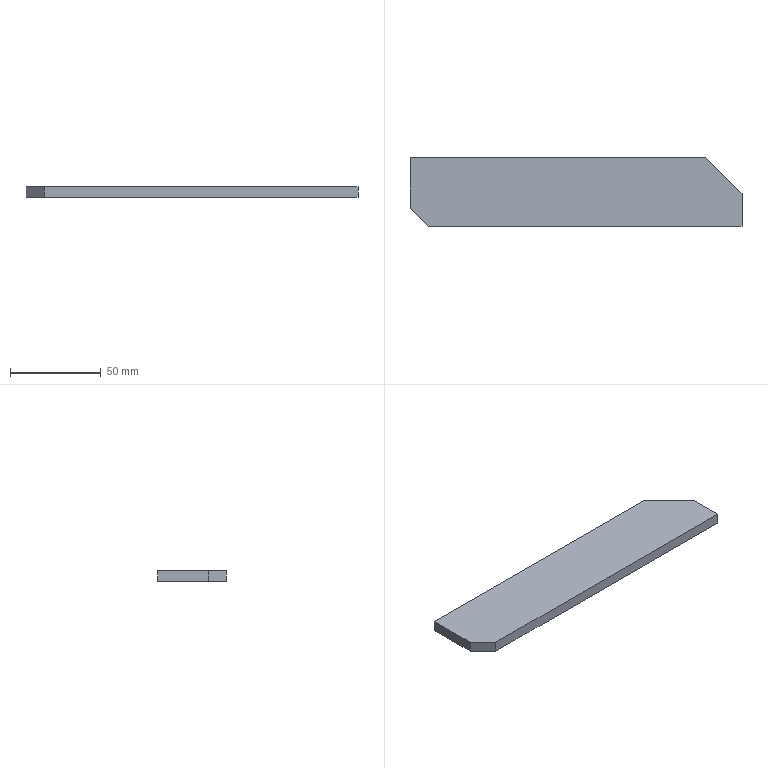Part | STEP file | [03]-10 | 1 solid | 8 faces | box 183 x 38 x 6 mm | volume 40224 mm3 | plane 8
STEP:
#1=CARTESIAN_POINT('',(0.,0.,0.));
#2=DIRECTION('',(0.,0.,1.));
#3=DIRECTION('',(1.,0.,0.));
#4=AXIS2_PLACEMENT_3D('',#1,#2,#3);
#5=CARTESIAN_POINT('',(0.,10.,6.));
#6=VERTEX_POINT('',#5);
#7=CARTESIAN_POINT('',(0.,38.,6.));
#8=VERTEX_POINT('',#7);
#9=CARTESIAN_POINT('',(0.,19.,6.));
#10=DIRECTION('',(0.,1.,0.));
#11=VECTOR('',#10,1.);
#12=LINE('',#9,#11);
#13=CARTESIAN_POINT('',(91.5,19.,6.));
#14=DIRECTION('',(0.,0.,1.));
#15=DIRECTION('',(-1.,0.,0.));
#16=AXIS2_PLACEMENT_3D('',#13,#14,#15);
#17=PLANE('',#16);
#18=CARTESIAN_POINT('',(91.5,0.));
#19=DIRECTION('',(0.,-1.));
#20=VECTOR('',#19,1.);
#21=LINE('',#18,#20);
#22=(GEOMETRIC_REPRESENTATION_CONTEXT(2)PARAMETRIC_REPRESENTATION_CONTEXT()REPRESENTATION_CONTEXT('',''));
#23=DEFINITIONAL_REPRESENTATION('',(#21),#22);
#24=PCURVE('',#17,#23);
#25=CARTESIAN_POINT('',(0.,19.,0.));
#26=DIRECTION('',(-1.,0.,0.));
#27=DIRECTION('',(0.,0.,-1.));
#28=AXIS2_PLACEMENT_3D('',#25,#26,#27);
#29=PLANE('',#28);
#30=CARTESIAN_POINT('',(-6.,0.));
#31=DIRECTION('',(0.,-1.));
#32=VECTOR('',#31,1.);
#33=LINE('',#30,#32);
#34=(GEOMETRIC_REPRESENTATION_CONTEXT(2)PARAMETRIC_REPRESENTATION_CONTEXT()REPRESENTATION_CONTEXT('',''));
#35=DEFINITIONAL_REPRESENTATION('',(#33),#34);
#36=PCURVE('',#29,#35);
#37=SURFACE_CURVE('',#12,(#24,#36),.PCURVE_S1.);
#38=EDGE_CURVE('',#6,#8,#37,.T.);
#39=ORIENTED_EDGE('',*,*,#38,.F.);
#40=CARTESIAN_POINT('',(10.,0.,6.));
#41=VERTEX_POINT('',#40);
#42=CARTESIAN_POINT('',(41.25,-31.25,6.));
#43=DIRECTION('',(0.7071,-0.7071,0.));
#44=VECTOR('',#43,1.);
#45=LINE('',#42,#44);
#46=CARTESIAN_POINT('',(50.25,50.25));
#47=DIRECTION('',(-0.7071,0.7071));
#48=VECTOR('',#47,1.);
#49=LINE('',#46,#48);
#50=(GEOMETRIC_REPRESENTATION_CONTEXT(2)PARAMETRIC_REPRESENTATION_CONTEXT()REPRESENTATION_CONTEXT('',''));
#51=DEFINITIONAL_REPRESENTATION('',(#49),#50);
#52=PCURVE('',#17,#51);
#53=CARTESIAN_POINT('',(0.,10.,0.));
#54=DIRECTION('',(0.7071,0.7071,0.));
#55=DIRECTION('',(0.,0.,1.));
#56=AXIS2_PLACEMENT_3D('',#53,#54,#55);
#57=PLANE('',#56);
#58=CARTESIAN_POINT('',(6.,58.336));
#59=DIRECTION('',(0.,1.));
#60=VECTOR('',#59,1.);
#61=LINE('',#58,#60);
#62=(GEOMETRIC_REPRESENTATION_CONTEXT(2)PARAMETRIC_REPRESENTATION_CONTEXT()REPRESENTATION_CONTEXT('',''));
#63=DEFINITIONAL_REPRESENTATION('',(#61),#62);
#64=PCURVE('',#57,#63);
#65=SURFACE_CURVE('',#45,(#52,#64),.PCURVE_S1.);
#66=EDGE_CURVE('',#6,#41,#65,.T.);
#67=ORIENTED_EDGE('',*,*,#66,.T.);
#68=CARTESIAN_POINT('',(183.,0.,6.));
#69=VERTEX_POINT('',#68);
#70=CARTESIAN_POINT('',(91.5,0.,6.));
#71=DIRECTION('',(-1.,0.,0.));
#72=VECTOR('',#71,1.);
#73=LINE('',#70,#72);
#74=CARTESIAN_POINT('',(0.,19.));
#75=DIRECTION('',(1.,0.));
#76=VECTOR('',#75,1.);
#77=LINE('',#74,#76);
#78=(GEOMETRIC_REPRESENTATION_CONTEXT(2)PARAMETRIC_REPRESENTATION_CONTEXT()REPRESENTATION_CONTEXT('',''));
#79=DEFINITIONAL_REPRESENTATION('',(#77),#78);
#80=PCURVE('',#17,#79);
#81=CARTESIAN_POINT('',(91.5,0.,0.));
#82=DIRECTION('',(0.,-1.,0.));
#83=DIRECTION('',(0.,0.,1.));
#84=AXIS2_PLACEMENT_3D('',#81,#82,#83);
#85=PLANE('',#84);
#86=CARTESIAN_POINT('',(6.,0.));
#87=DIRECTION('',(0.,1.));
#88=VECTOR('',#87,1.);
#89=LINE('',#86,#88);
#90=(GEOMETRIC_REPRESENTATION_CONTEXT(2)PARAMETRIC_REPRESENTATION_CONTEXT()REPRESENTATION_CONTEXT('',''));
#91=DEFINITIONAL_REPRESENTATION('',(#89),#90);
#92=PCURVE('',#85,#91);
#93=SURFACE_CURVE('',#73,(#80,#92),.PCURVE_S1.);
#94=EDGE_CURVE('',#69,#41,#93,.T.);
#95=ORIENTED_EDGE('',*,*,#94,.F.);
#96=CARTESIAN_POINT('',(183.,18.,6.));
#97=VERTEX_POINT('',#96);
#98=CARTESIAN_POINT('',(183.,19.,6.));
#99=DIRECTION('',(0.,-1.,0.));
#100=VECTOR('',#99,1.);
#101=LINE('',#98,#100);
#102=CARTESIAN_POINT('',(-91.5,0.));
#103=DIRECTION('',(0.,1.));
#104=VECTOR('',#103,1.);
#105=LINE('',#102,#104);
#106=(GEOMETRIC_REPRESENTATION_CONTEXT(2)PARAMETRIC_REPRESENTATION_CONTEXT()REPRESENTATION_CONTEXT('',''));
#107=DEFINITIONAL_REPRESENTATION('',(#105),#106);
#108=PCURVE('',#17,#107);
#109=CARTESIAN_POINT('',(183.,19.,0.));
#110=DIRECTION('',(1.,0.,0.));
#111=DIRECTION('',(0.,0.,1.));
#112=AXIS2_PLACEMENT_3D('',#109,#110,#111);
#113=PLANE('',#112);
#114=CARTESIAN_POINT('',(6.,0.));
#115=DIRECTION('',(0.,1.));
#116=VECTOR('',#115,1.);
#117=LINE('',#114,#116);
#118=(GEOMETRIC_REPRESENTATION_CONTEXT(2)PARAMETRIC_REPRESENTATION_CONTEXT()REPRESENTATION_CONTEXT('',''));
#119=DEFINITIONAL_REPRESENTATION('',(#117),#118);
#120=PCURVE('',#113,#119);
#121=SURFACE_CURVE('',#101,(#108,#120),.PCURVE_S1.);
#122=EDGE_CURVE('',#97,#69,#121,.T.);
#123=ORIENTED_EDGE('',*,*,#122,.F.);
#124=CARTESIAN_POINT('',(163.,38.,6.));
#125=VERTEX_POINT('',#124);
#126=CARTESIAN_POINT('',(136.75,64.25,6.));
#127=DIRECTION('',(-0.7071,0.7071,0.));
#128=VECTOR('',#127,1.);
#129=LINE('',#126,#128);
#130=CARTESIAN_POINT('',(-45.25,-45.25));
#131=DIRECTION('',(0.7071,-0.7071));
#132=VECTOR('',#131,1.);
#133=LINE('',#130,#132);
#134=(GEOMETRIC_REPRESENTATION_CONTEXT(2)PARAMETRIC_REPRESENTATION_CONTEXT()REPRESENTATION_CONTEXT('',''));
#135=DEFINITIONAL_REPRESENTATION('',(#133),#134);
#136=PCURVE('',#17,#135);
#137=CARTESIAN_POINT('',(183.,18.,0.));
#138=DIRECTION('',(-0.7071,-0.7071,0.));
#139=DIRECTION('',(0.,0.,1.));
#140=AXIS2_PLACEMENT_3D('',#137,#138,#139);
#141=PLANE('',#140);
#142=CARTESIAN_POINT('',(6.,65.407));
#143=DIRECTION('',(0.,1.));
#144=VECTOR('',#143,1.);
#145=LINE('',#142,#144);
#146=(GEOMETRIC_REPRESENTATION_CONTEXT(2)PARAMETRIC_REPRESENTATION_CONTEXT()REPRESENTATION_CONTEXT('',''));
#147=DEFINITIONAL_REPRESENTATION('',(#145),#146);
#148=PCURVE('',#141,#147);
#149=SURFACE_CURVE('',#129,(#136,#148),.PCURVE_S1.);
#150=EDGE_CURVE('',#97,#125,#149,.T.);
#151=ORIENTED_EDGE('',*,*,#150,.T.);
#152=CARTESIAN_POINT('',(91.5,38.,6.));
#153=DIRECTION('',(1.,0.,0.));
#154=VECTOR('',#153,1.);
#155=LINE('',#152,#154);
#156=CARTESIAN_POINT('',(0.,-19.));
#157=DIRECTION('',(-1.,0.));
#158=VECTOR('',#157,1.);
#159=LINE('',#156,#158);
#160=(GEOMETRIC_REPRESENTATION_CONTEXT(2)PARAMETRIC_REPRESENTATION_CONTEXT()REPRESENTATION_CONTEXT('',''));
#161=DEFINITIONAL_REPRESENTATION('',(#159),#160);
#162=PCURVE('',#17,#161);
#163=CARTESIAN_POINT('',(91.5,38.,0.));
#164=DIRECTION('',(0.,1.,0.));
#165=DIRECTION('',(0.,0.,-1.));
#166=AXIS2_PLACEMENT_3D('',#163,#164,#165);
#167=PLANE('',#166);
#168=CARTESIAN_POINT('',(-6.,0.));
#169=DIRECTION('',(0.,-1.));
#170=VECTOR('',#169,1.);
#171=LINE('',#168,#170);
#172=(GEOMETRIC_REPRESENTATION_CONTEXT(2)PARAMETRIC_REPRESENTATION_CONTEXT()REPRESENTATION_CONTEXT('',''));
#173=DEFINITIONAL_REPRESENTATION('',(#171),#172);
#174=PCURVE('',#167,#173);
#175=SURFACE_CURVE('',#155,(#162,#174),.PCURVE_S1.);
#176=EDGE_CURVE('',#8,#125,#175,.T.);
#177=ORIENTED_EDGE('',*,*,#176,.F.);
#178=EDGE_LOOP('',(#39,#67,#95,#123,#151,#177));
#179=FACE_BOUND('',#178,.T.);
#180=ADVANCED_FACE('',(#179),#17,.T.);
#181=ORIENTED_EDGE('',*,*,#176,.T.);
#182=CARTESIAN_POINT('',(163.,38.,0.));
#183=VERTEX_POINT('',#182);
#184=CARTESIAN_POINT('',(163.,38.,0.));
#185=DIRECTION('',(0.,0.,-1.));
#186=VECTOR('',#185,1.);
#187=LINE('',#184,#186);
#188=CARTESIAN_POINT('',(0.,-71.5));
#189=DIRECTION('',(1.,0.));
#190=VECTOR('',#189,1.);
#191=LINE('',#188,#190);
#192=(GEOMETRIC_REPRESENTATION_CONTEXT(2)PARAMETRIC_REPRESENTATION_CONTEXT()REPRESENTATION_CONTEXT('',''));
#193=DEFINITIONAL_REPRESENTATION('',(#191),#192);
#194=PCURVE('',#167,#193);
#195=CARTESIAN_POINT('',(0.,28.284));
#196=DIRECTION('',(-1.,0.));
#197=VECTOR('',#196,1.);
#198=LINE('',#195,#197);
#199=(GEOMETRIC_REPRESENTATION_CONTEXT(2)PARAMETRIC_REPRESENTATION_CONTEXT()REPRESENTATION_CONTEXT('',''));
#200=DEFINITIONAL_REPRESENTATION('',(#198),#199);
#201=PCURVE('',#141,#200);
#202=SURFACE_CURVE('',#187,(#194,#201),.PCURVE_S1.);
#203=EDGE_CURVE('',#125,#183,#202,.T.);
#204=ORIENTED_EDGE('',*,*,#203,.T.);
#205=CARTESIAN_POINT('',(0.,38.,0.));
#206=VERTEX_POINT('',#205);
#207=CARTESIAN_POINT('',(91.5,38.,0.));
#208=DIRECTION('',(-1.,0.,0.));
#209=VECTOR('',#208,1.);
#210=LINE('',#207,#209);
#211=CARTESIAN_POINT('',(0.,0.));
#212=DIRECTION('',(0.,1.));
#213=VECTOR('',#212,1.);
#214=LINE('',#211,#213);
#215=(GEOMETRIC_REPRESENTATION_CONTEXT(2)PARAMETRIC_REPRESENTATION_CONTEXT()REPRESENTATION_CONTEXT('',''));
#216=DEFINITIONAL_REPRESENTATION('',(#214),#215);
#217=PCURVE('',#167,#216);
#218=CARTESIAN_POINT('',(91.5,19.,0.));
#219=DIRECTION('',(0.,0.,-1.));
#220=DIRECTION('',(1.,0.,0.));
#221=AXIS2_PLACEMENT_3D('',#218,#219,#220);
#222=PLANE('',#221);
#223=CARTESIAN_POINT('',(0.,-19.));
#224=DIRECTION('',(-1.,0.));
#225=VECTOR('',#224,1.);
#226=LINE('',#223,#225);
#227=(GEOMETRIC_REPRESENTATION_CONTEXT(2)PARAMETRIC_REPRESENTATION_CONTEXT()REPRESENTATION_CONTEXT('',''));
#228=DEFINITIONAL_REPRESENTATION('',(#226),#227);
#229=PCURVE('',#222,#228);
#230=SURFACE_CURVE('',#210,(#217,#229),.PCURVE_S1.);
#231=EDGE_CURVE('',#183,#206,#230,.T.);
#232=ORIENTED_EDGE('',*,*,#231,.T.);
#233=CARTESIAN_POINT('',(0.,38.,0.));
#234=DIRECTION('',(0.,0.,1.));
#235=VECTOR('',#234,1.);
#236=LINE('',#233,#235);
#237=CARTESIAN_POINT('',(0.,91.5));
#238=DIRECTION('',(-1.,0.));
#239=VECTOR('',#238,1.);
#240=LINE('',#237,#239);
#241=(GEOMETRIC_REPRESENTATION_CONTEXT(2)PARAMETRIC_REPRESENTATION_CONTEXT()REPRESENTATION_CONTEXT('',''));
#242=DEFINITIONAL_REPRESENTATION('',(#240),#241);
#243=PCURVE('',#167,#242);
#244=CARTESIAN_POINT('',(0.,-19.));
#245=DIRECTION('',(-1.,0.));
#246=VECTOR('',#245,1.);
#247=LINE('',#244,#246);
#248=(GEOMETRIC_REPRESENTATION_CONTEXT(2)PARAMETRIC_REPRESENTATION_CONTEXT()REPRESENTATION_CONTEXT('',''));
#249=DEFINITIONAL_REPRESENTATION('',(#247),#248);
#250=PCURVE('',#29,#249);
#251=SURFACE_CURVE('',#236,(#243,#250),.PCURVE_S1.);
#252=EDGE_CURVE('',#206,#8,#251,.T.);
#253=ORIENTED_EDGE('',*,*,#252,.T.);
#254=EDGE_LOOP('',(#181,#204,#232,#253));
#255=FACE_BOUND('',#254,.T.);
#256=ADVANCED_FACE('',(#255),#167,.T.);
#257=CARTESIAN_POINT('',(183.,0.,0.));
#258=VERTEX_POINT('',#257);
#259=CARTESIAN_POINT('',(183.,18.,0.));
#260=VERTEX_POINT('',#259);
#261=CARTESIAN_POINT('',(183.,19.,0.));
#262=DIRECTION('',(0.,1.,0.));
#263=VECTOR('',#262,1.);
#264=LINE('',#261,#263);
#265=CARTESIAN_POINT('',(0.,0.));
#266=DIRECTION('',(0.,-1.));
#267=VECTOR('',#266,1.);
#268=LINE('',#265,#267);
#269=(GEOMETRIC_REPRESENTATION_CONTEXT(2)PARAMETRIC_REPRESENTATION_CONTEXT()REPRESENTATION_CONTEXT('',''));
#270=DEFINITIONAL_REPRESENTATION('',(#268),#269);
#271=PCURVE('',#113,#270);
#272=CARTESIAN_POINT('',(91.5,0.));
#273=DIRECTION('',(0.,-1.));
#274=VECTOR('',#273,1.);
#275=LINE('',#272,#274);
#276=(GEOMETRIC_REPRESENTATION_CONTEXT(2)PARAMETRIC_REPRESENTATION_CONTEXT()REPRESENTATION_CONTEXT('',''));
#277=DEFINITIONAL_REPRESENTATION('',(#275),#276);
#278=PCURVE('',#222,#277);
#279=SURFACE_CURVE('',#264,(#271,#278),.PCURVE_S1.);
#280=EDGE_CURVE('',#258,#260,#279,.T.);
#281=ORIENTED_EDGE('',*,*,#280,.T.);
#282=CARTESIAN_POINT('',(183.,18.,0.));
#283=DIRECTION('',(0.,0.,1.));
#284=VECTOR('',#283,1.);
#285=LINE('',#282,#284);
#286=CARTESIAN_POINT('',(0.,1.));
#287=DIRECTION('',(1.,0.));
#288=VECTOR('',#287,1.);
#289=LINE('',#286,#288);
#290=(GEOMETRIC_REPRESENTATION_CONTEXT(2)PARAMETRIC_REPRESENTATION_CONTEXT()REPRESENTATION_CONTEXT('',''));
#291=DEFINITIONAL_REPRESENTATION('',(#289),#290);
#292=PCURVE('',#113,#291);
#293=CARTESIAN_POINT('',(0.,0.));
#294=DIRECTION('',(1.,0.));
#295=VECTOR('',#294,1.);
#296=LINE('',#293,#295);
#297=(GEOMETRIC_REPRESENTATION_CONTEXT(2)PARAMETRIC_REPRESENTATION_CONTEXT()REPRESENTATION_CONTEXT('',''));
#298=DEFINITIONAL_REPRESENTATION('',(#296),#297);
#299=PCURVE('',#141,#298);
#300=SURFACE_CURVE('',#285,(#292,#299),.PCURVE_S1.);
#301=EDGE_CURVE('',#260,#97,#300,.T.);
#302=ORIENTED_EDGE('',*,*,#301,.T.);
#303=ORIENTED_EDGE('',*,*,#122,.T.);
#304=CARTESIAN_POINT('',(183.,0.,0.));
#305=DIRECTION('',(0.,0.,1.));
#306=VECTOR('',#305,1.);
#307=LINE('',#304,#306);
#308=CARTESIAN_POINT('',(0.,19.));
#309=DIRECTION('',(1.,0.));
#310=VECTOR('',#309,1.);
#311=LINE('',#308,#310);
#312=(GEOMETRIC_REPRESENTATION_CONTEXT(2)PARAMETRIC_REPRESENTATION_CONTEXT()REPRESENTATION_CONTEXT('',''));
#313=DEFINITIONAL_REPRESENTATION('',(#311),#312);
#314=PCURVE('',#113,#313);
#315=CARTESIAN_POINT('',(0.,-91.5));
#316=DIRECTION('',(1.,0.));
#317=VECTOR('',#316,1.);
#318=LINE('',#315,#317);
#319=(GEOMETRIC_REPRESENTATION_CONTEXT(2)PARAMETRIC_REPRESENTATION_CONTEXT()REPRESENTATION_CONTEXT('',''));
#320=DEFINITIONAL_REPRESENTATION('',(#318),#319);
#321=PCURVE('',#85,#320);
#322=SURFACE_CURVE('',#307,(#314,#321),.PCURVE_S1.);
#323=EDGE_CURVE('',#258,#69,#322,.T.);
#324=ORIENTED_EDGE('',*,*,#323,.F.);
#325=EDGE_LOOP('',(#281,#302,#303,#324));
#326=FACE_BOUND('',#325,.T.);
#327=ADVANCED_FACE('',(#326),#113,.T.);
#328=ORIENTED_EDGE('',*,*,#94,.T.);
#329=CARTESIAN_POINT('',(10.,0.,0.));
#330=VERTEX_POINT('',#329);
#331=CARTESIAN_POINT('',(10.,0.,0.));
#332=DIRECTION('',(0.,0.,-1.));
#333=VECTOR('',#332,1.);
#334=LINE('',#331,#333);
#335=CARTESIAN_POINT('',(0.,81.5));
#336=DIRECTION('',(-1.,0.));
#337=VECTOR('',#336,1.);
#338=LINE('',#335,#337);
#339=(GEOMETRIC_REPRESENTATION_CONTEXT(2)PARAMETRIC_REPRESENTATION_CONTEXT()REPRESENTATION_CONTEXT('',''));
#340=DEFINITIONAL_REPRESENTATION('',(#338),#339);
#341=PCURVE('',#85,#340);
#342=CARTESIAN_POINT('',(0.,14.142));
#343=DIRECTION('',(-1.,0.));
#344=VECTOR('',#343,1.);
#345=LINE('',#342,#344);
#346=(GEOMETRIC_REPRESENTATION_CONTEXT(2)PARAMETRIC_REPRESENTATION_CONTEXT()REPRESENTATION_CONTEXT('',''));
#347=DEFINITIONAL_REPRESENTATION('',(#345),#346);
#348=PCURVE('',#57,#347);
#349=SURFACE_CURVE('',#334,(#341,#348),.PCURVE_S1.);
#350=EDGE_CURVE('',#41,#330,#349,.T.);
#351=ORIENTED_EDGE('',*,*,#350,.T.);
#352=CARTESIAN_POINT('',(91.5,0.,0.));
#353=DIRECTION('',(1.,0.,0.));
#354=VECTOR('',#353,1.);
#355=LINE('',#352,#354);
#356=CARTESIAN_POINT('',(0.,0.));
#357=DIRECTION('',(0.,-1.));
#358=VECTOR('',#357,1.);
#359=LINE('',#356,#358);
#360=(GEOMETRIC_REPRESENTATION_CONTEXT(2)PARAMETRIC_REPRESENTATION_CONTEXT()REPRESENTATION_CONTEXT('',''));
#361=DEFINITIONAL_REPRESENTATION('',(#359),#360);
#362=PCURVE('',#85,#361);
#363=CARTESIAN_POINT('',(0.,19.));
#364=DIRECTION('',(1.,0.));
#365=VECTOR('',#364,1.);
#366=LINE('',#363,#365);
#367=(GEOMETRIC_REPRESENTATION_CONTEXT(2)PARAMETRIC_REPRESENTATION_CONTEXT()REPRESENTATION_CONTEXT('',''));
#368=DEFINITIONAL_REPRESENTATION('',(#366),#367);
#369=PCURVE('',#222,#368);
#370=SURFACE_CURVE('',#355,(#362,#369),.PCURVE_S1.);
#371=EDGE_CURVE('',#330,#258,#370,.T.);
#372=ORIENTED_EDGE('',*,*,#371,.T.);
#373=ORIENTED_EDGE('',*,*,#323,.T.);
#374=EDGE_LOOP('',(#328,#351,#372,#373));
#375=FACE_BOUND('',#374,.T.);
#376=ADVANCED_FACE('',(#375),#85,.T.);
#377=ORIENTED_EDGE('',*,*,#371,.F.);
#378=CARTESIAN_POINT('',(0.,10.,0.));
#379=VERTEX_POINT('',#378);
#380=CARTESIAN_POINT('',(41.25,-31.25,0.));
#381=DIRECTION('',(-0.7071,0.7071,0.));
#382=VECTOR('',#381,1.);
#383=LINE('',#380,#382);
#384=CARTESIAN_POINT('',(-50.25,50.25));
#385=DIRECTION('',(-0.7071,-0.7071));
#386=VECTOR('',#385,1.);
#387=LINE('',#384,#386);
#388=(GEOMETRIC_REPRESENTATION_CONTEXT(2)PARAMETRIC_REPRESENTATION_CONTEXT()REPRESENTATION_CONTEXT('',''));
#389=DEFINITIONAL_REPRESENTATION('',(#387),#388);
#390=PCURVE('',#222,#389);
#391=CARTESIAN_POINT('',(0.,58.336));
#392=DIRECTION('',(0.,-1.));
#393=VECTOR('',#392,1.);
#394=LINE('',#391,#393);
#395=(GEOMETRIC_REPRESENTATION_CONTEXT(2)PARAMETRIC_REPRESENTATION_CONTEXT()REPRESENTATION_CONTEXT('',''));
#396=DEFINITIONAL_REPRESENTATION('',(#394),#395);
#397=PCURVE('',#57,#396);
#398=SURFACE_CURVE('',#383,(#390,#397),.PCURVE_S1.);
#399=EDGE_CURVE('',#330,#379,#398,.T.);
#400=ORIENTED_EDGE('',*,*,#399,.T.);
#401=CARTESIAN_POINT('',(0.,19.,0.));
#402=DIRECTION('',(0.,-1.,0.));
#403=VECTOR('',#402,1.);
#404=LINE('',#401,#403);
#405=CARTESIAN_POINT('',(-91.5,0.));
#406=DIRECTION('',(0.,1.));
#407=VECTOR('',#406,1.);
#408=LINE('',#405,#407);
#409=(GEOMETRIC_REPRESENTATION_CONTEXT(2)PARAMETRIC_REPRESENTATION_CONTEXT()REPRESENTATION_CONTEXT('',''));
#410=DEFINITIONAL_REPRESENTATION('',(#408),#409);
#411=PCURVE('',#222,#410);
#412=CARTESIAN_POINT('',(0.,0.));
#413=DIRECTION('',(0.,1.));
#414=VECTOR('',#413,1.);
#415=LINE('',#412,#414);
#416=(GEOMETRIC_REPRESENTATION_CONTEXT(2)PARAMETRIC_REPRESENTATION_CONTEXT()REPRESENTATION_CONTEXT('',''));
#417=DEFINITIONAL_REPRESENTATION('',(#415),#416);
#418=PCURVE('',#29,#417);
#419=SURFACE_CURVE('',#404,(#411,#418),.PCURVE_S1.);
#420=EDGE_CURVE('',#206,#379,#419,.T.);
#421=ORIENTED_EDGE('',*,*,#420,.F.);
#422=ORIENTED_EDGE('',*,*,#231,.F.);
#423=CARTESIAN_POINT('',(136.75,64.25,0.));
#424=DIRECTION('',(0.7071,-0.7071,0.));
#425=VECTOR('',#424,1.);
#426=LINE('',#423,#425);
#427=CARTESIAN_POINT('',(45.25,-45.25));
#428=DIRECTION('',(0.7071,0.7071));
#429=VECTOR('',#428,1.);
#430=LINE('',#427,#429);
#431=(GEOMETRIC_REPRESENTATION_CONTEXT(2)PARAMETRIC_REPRESENTATION_CONTEXT()REPRESENTATION_CONTEXT('',''));
#432=DEFINITIONAL_REPRESENTATION('',(#430),#431);
#433=PCURVE('',#222,#432);
#434=CARTESIAN_POINT('',(0.,65.407));
#435=DIRECTION('',(0.,-1.));
#436=VECTOR('',#435,1.);
#437=LINE('',#434,#436);
#438=(GEOMETRIC_REPRESENTATION_CONTEXT(2)PARAMETRIC_REPRESENTATION_CONTEXT()REPRESENTATION_CONTEXT('',''));
#439=DEFINITIONAL_REPRESENTATION('',(#437),#438);
#440=PCURVE('',#141,#439);
#441=SURFACE_CURVE('',#426,(#433,#440),.PCURVE_S1.);
#442=EDGE_CURVE('',#183,#260,#441,.T.);
#443=ORIENTED_EDGE('',*,*,#442,.T.);
#444=ORIENTED_EDGE('',*,*,#280,.F.);
#445=EDGE_LOOP('',(#377,#400,#421,#422,#443,#444));
#446=FACE_BOUND('',#445,.T.);
#447=ADVANCED_FACE('',(#446),#222,.T.);
#448=ORIENTED_EDGE('',*,*,#420,.T.);
#449=CARTESIAN_POINT('',(0.,10.,0.));
#450=DIRECTION('',(0.,0.,1.));
#451=VECTOR('',#450,1.);
#452=LINE('',#449,#451);
#453=CARTESIAN_POINT('',(0.,9.));
#454=DIRECTION('',(-1.,0.));
#455=VECTOR('',#454,1.);
#456=LINE('',#453,#455);
#457=(GEOMETRIC_REPRESENTATION_CONTEXT(2)PARAMETRIC_REPRESENTATION_CONTEXT()REPRESENTATION_CONTEXT('',''));
#458=DEFINITIONAL_REPRESENTATION('',(#456),#457);
#459=PCURVE('',#29,#458);
#460=CARTESIAN_POINT('',(0.,0.));
#461=DIRECTION('',(1.,0.));
#462=VECTOR('',#461,1.);
#463=LINE('',#460,#462);
#464=(GEOMETRIC_REPRESENTATION_CONTEXT(2)PARAMETRIC_REPRESENTATION_CONTEXT()REPRESENTATION_CONTEXT('',''));
#465=DEFINITIONAL_REPRESENTATION('',(#463),#464);
#466=PCURVE('',#57,#465);
#467=SURFACE_CURVE('',#452,(#459,#466),.PCURVE_S1.);
#468=EDGE_CURVE('',#379,#6,#467,.T.);
#469=ORIENTED_EDGE('',*,*,#468,.T.);
#470=ORIENTED_EDGE('',*,*,#38,.T.);
#471=ORIENTED_EDGE('',*,*,#252,.F.);
#472=EDGE_LOOP('',(#448,#469,#470,#471));
#473=FACE_BOUND('',#472,.T.);
#474=ADVANCED_FACE('',(#473),#29,.T.);
#475=ORIENTED_EDGE('',*,*,#442,.F.);
#476=ORIENTED_EDGE('',*,*,#203,.F.);
#477=ORIENTED_EDGE('',*,*,#150,.F.);
#478=ORIENTED_EDGE('',*,*,#301,.F.);
#479=EDGE_LOOP('',(#475,#476,#477,#478));
#480=FACE_BOUND('',#479,.T.);
#481=ADVANCED_FACE('',(#480),#141,.F.);
#482=ORIENTED_EDGE('',*,*,#399,.F.);
#483=ORIENTED_EDGE('',*,*,#350,.F.);
#484=ORIENTED_EDGE('',*,*,#66,.F.);
#485=ORIENTED_EDGE('',*,*,#468,.F.);
#486=EDGE_LOOP('',(#482,#483,#484,#485));
#487=FACE_BOUND('',#486,.T.);
#488=ADVANCED_FACE('',(#487),#57,.F.);
#489=CLOSED_SHELL('',(#180,#256,#327,#376,#447,#474,#481,#488));
#490=MANIFOLD_SOLID_BREP('',#489);
#491=(LENGTH_UNIT()NAMED_UNIT(*)SI_UNIT(.MILLI.,.METRE.));
#492=UNCERTAINTY_MEASURE_WITH_UNIT(LENGTH_MEASURE(0.0000001),#491,'','');
#493=(NAMED_UNIT(*)PLANE_ANGLE_UNIT()SI_UNIT($,.RADIAN.));
#494=(NAMED_UNIT(*)SI_UNIT($,.STERADIAN.)SOLID_ANGLE_UNIT());
#495=(GEOMETRIC_REPRESENTATION_CONTEXT(3)GLOBAL_UNCERTAINTY_ASSIGNED_CONTEXT((#492))GLOBAL_UNIT_ASSIGNED_CONTEXT((#491,#493,#494))REPRESENTATION_CONTEXT('',''));
#496=ADVANCED_BREP_SHAPE_REPRESENTATION('',(#4,#490),#495);